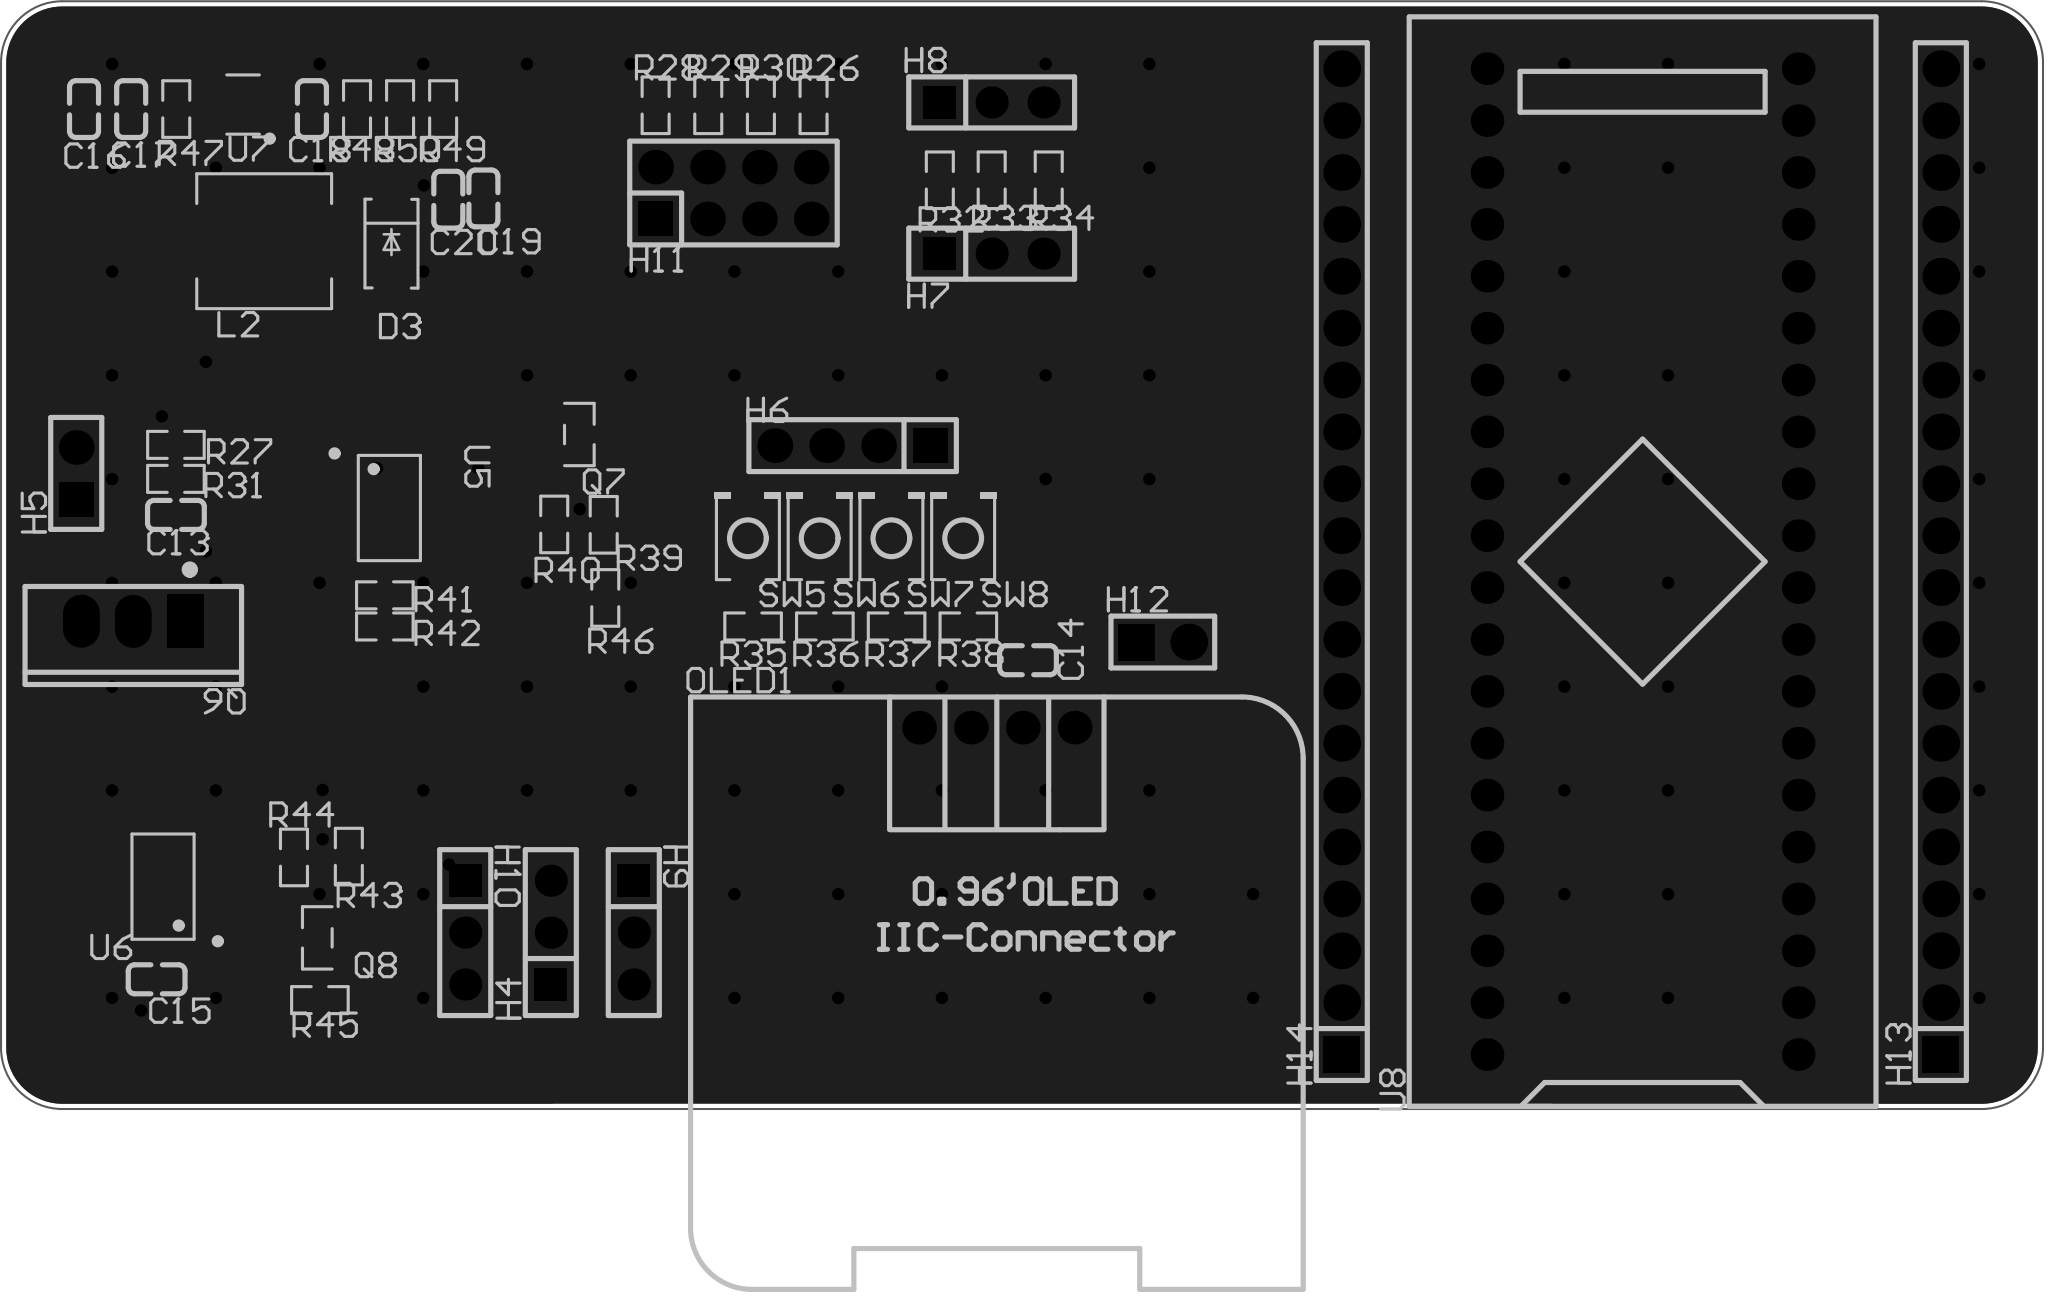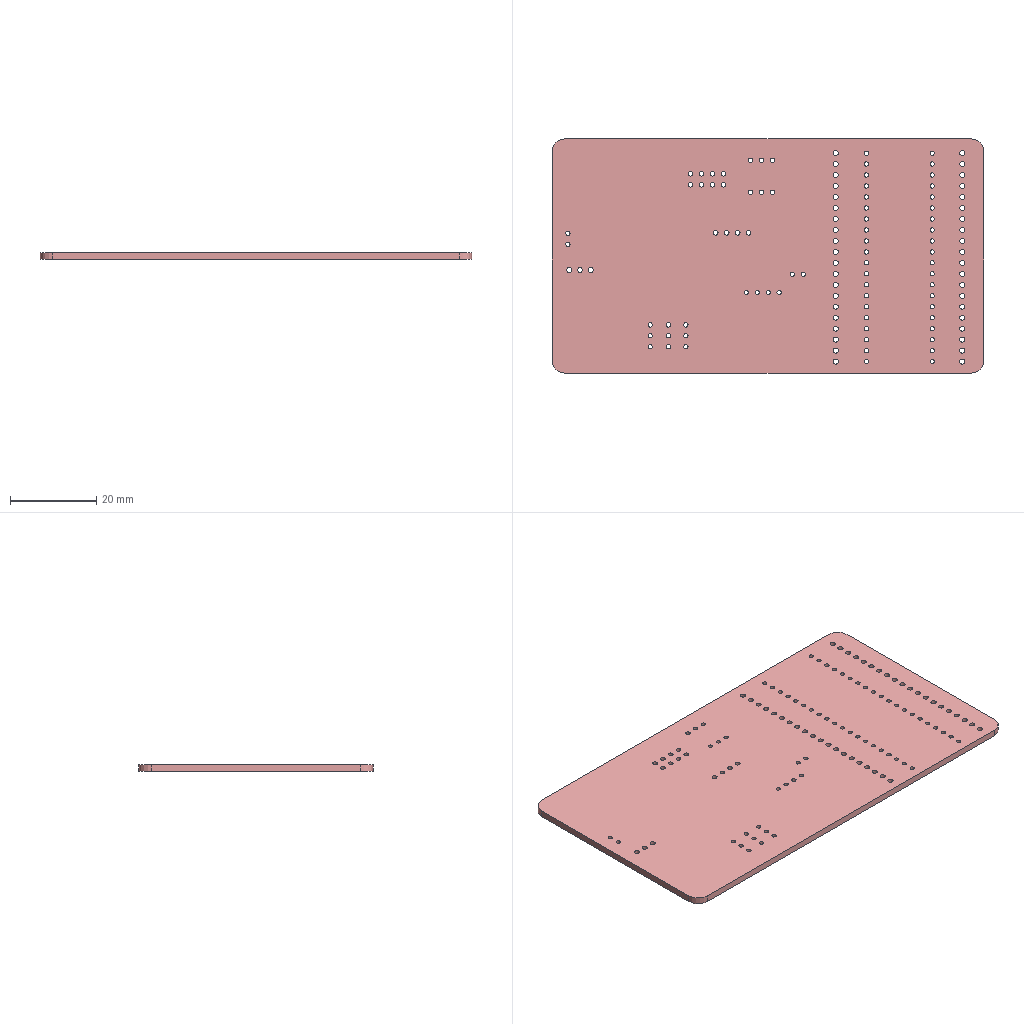Circuit board layout | Altium Designer | box 100 x 54.2 x 1.6 mm
Layer stack:
# Altium Designer layer stack of  (unit mm; dielectric type: 0 none, 1 core, 2 prepreg, 3 surface material)
index,name,kind,layer,copper_thickness_mm,dielectric_type,dielectric_thickness_mm,dielectric_material,dielectric_constant
0,Top Paste Mask Layer,other,,,,,,
1,Top Silkscreen Layer,other,,,,,,
2,Top Solder Mask Layer,dielectric,,,3,0.01,,3.3
3,Top Layer,copper,Top Layer,0.035,,,,
4,Dielectric1,dielectric,,,3,1.51,FR4,4.5
5,Bottom Layer,copper,Bottom Layer,0.035,,,,
6,Bottom Solder Mask Layer,dielectric,,,3,0.01,,3.3
7,Bottom Silkscreen Layer,other,,,,,,
8,Bottom Paste Mask Layer,other,,,,,,
# drill layer pairs: low layer,high layer
drill_pair,Top Layer,Bottom Layer
Part placement:
Designator,Comment,Layer,Footprint,Center-X(mm),Center-Y(mm),Rotation
C13,104,TopLayer,C0603,87.178,114.214,0
C14,10uf,TopLayer,C0603,128.905,107.102,180
C15,100nF,TopLayer,C0603,86.233,91.481,180
C16,106,TopLayer,C0603,82.677,134.082,90
C17,104,TopLayer,C0603,84.986,134.082,90
C18,100pF,TopLayer,C0603,93.838,134.082,90
C19,10UF,TopLayer,C0603,102.235,129.708,270
C20,104,TopLayer,C0603,100.517,129.645,270
D3,SS36,TopLayer,SMA_L4.3-W2.6-LS5.0-FD,97.723,127.487,90
H4,,TopLayer,HDR-TH_3P-P2.54-V-F,105.537,93.767,90
H5,,TopLayer,HDR-TH_2P-P2.54-V-F,82.296,116.246,90
H6,,TopLayer,HDR-TH_4P-P2.54-V-M,120.317,117.606,180
H7,,TopLayer,HDR-TH_3P-P2.54-V-F,127.127,127.004,0
H8,,TopLayer,HDR-TH_3P-P2.54-V-F,127.127,134.407,0
H9,,TopLayer,HDR-TH_3P-P2.54-V-F,109.601,93.767,270
H10,,TopLayer,HDR-TH_3P-P2.54-V-F,101.346,93.767,270
H11,,TopLayer,HDR-TH_8P-P2.54-V-M-R2-C4-S2.54,114.482,129.973,0
L2,22uH,TopLayer,IND-SMD_L7.1-W6.6,91.5,127.614,0
Q6,2N6804,TopLayer,TO-220-3_L10.0-W4.5-P2.54-L,85.09,109.007,180
Q7,SS8550,TopLayer,SOT-23-3_L2.9-W1.3-P1.90-LS2.4-BR,106.934,118.151,180
Q8,SS8550,TopLayer,SOT-23-3_L2.9-W1.3-P1.90-LS2.4-BR,94.102,93.509,0
R26,100K,TopLayer,R0603,118.404,134.267,90
R27,1K,TopLayer,R0603,87.178,117.643,180
R28,200,TopLayer,R0603,110.669,134.267,90
R29,2K,TopLayer,R0603,113.248,134.267,90
R30,20K,TopLayer,R0603,115.826,134.267,90
R31,1K,TopLayer,R0603,87.178,115.979,0
R32,100,TopLayer,R0603,124.587,130.597,270
R33,100,TopLayer,R0603,127.127,130.597,270
R34,100,TopLayer,R0603,129.921,130.597,90
R35,100,TopLayer,R0603,115.443,108.753,0
R36,100,TopLayer,R0603,118.957,108.753,0
R37,100,TopLayer,R0603,122.47,108.753,0
R38,100,TopLayer,R0603,125.984,108.753,0
R39,1K,TopLayer,R0603,108.127,113.731,90
R40,250K,TopLayer,R0603,105.704,113.748,90
R41,10K,TopLayer,R0603,97.409,110.277,180
R42,10K,TopLayer,R0603,97.409,108.753,0
R43,10K,TopLayer,R0603,95.646,97.487,90
R44,10K,TopLayer,R0603,92.959,97.446,270
R45,250K,TopLayer,R0603,94.229,90.461,0
R46,1K,TopLayer,R0603,108.204,110.15,270
R47,1K,TopLayer,R0603,87.195,134.082,270
R48,1K,TopLayer,R0603,96.047,134.082,90
R49,9.1K,TopLayer,R0603,100.263,134.082,90
R50,75K,TopLayer,R0603,98.155,134.082,90
SW5,TS-1088-AR02016,TopLayer,SW-SMD_L3.9-W3.0-P4.45,115.189,113.071,90
SW6,TS-1088-AR02016,TopLayer,SW-SMD_L3.9-W3.0-P4.45,118.703,113.071,90
SW7,TS-1088-AR02016,TopLayer,SW-SMD_L3.9-W3.0-P4.45,122.216,113.071,90
SW8,TS-1088-AR02016,TopLayer,SW-SMD_L3.9-W3.0-P4.45,125.73,113.071,90
U5,LM358DTR(XBLW),TopLayer,SOIC-8_L4.9-W4.0-P1.27-LS6.0-BL,97.63,114.552,270
U6,LM358DTR(XBLW),TopLayer,SOIC-8_L4.9-W4.0-P1.27-LS6.0-BL,86.546,96.017,90
U7,MT3608L,TopLayer,SOT-23-6_L2.9-W1.6-P0.95-LS2.8-BL_3,90.466,134.303,90
H12,,TopLayer,HDR-TH_2P-P2.54-V-M-1,135.509,107.991,0
U8,STM32F103C8T6-Card,TopLayer,CONN-TH_L53.3-W22.9_STM32F103C8T6-CARD,159.004,111.928,90
H13,,TopLayer,HDR-TH_20P-P2.54-V-M-1,173.609,111.928,90
H14,,TopLayer,HDR-TH_20P-P2.54-V-M-1,144.272,111.928,90
OLED1,,TopLayer,0.96OLED_4P,127.381,103.8,0
Pad and via stacks:
# Altium Designer via and pad stacks of  (unit mm). Each distinct definition once, with the count of objects using it.
# via: kind,start_layer,end_layer,hole_mm,diameter_mm,mode(0 simple;1 top-mid-bottom;2 full stack),diameter_per_layer,count,example_net
# pad: kind,layer,hole_mm,hole_type(0 round;1 square;2 slot),plating,top_size,top_shape(1 round;2 rect;3 octagon;9 rounded rect),mid_size,bottom_size,mode,footprint,size_per_layer,count,example
pad,Top Layer,0,0,plated,0.8x0.9,2,0.8x0.9,0.8x0.9,0,C0603,,16,C13.2
pad,Top Layer,0,0,plated,2.046x1.62,2,2.046x1.62,2.046x1.62,0,SMA_L4.3-W2.6-LS5.0-FD,,2,D3.1
pad,Top Layer,0,0,plated,2.15x3.32,2,2.15x3.32,2.15x3.32,0,IND-SMD_L7.1-W6.6,,2,L2.2
pad,Top Layer,0,0,plated,1.25x0.7,2,1.25x0.7,1.25x0.7,0,SOT-23-3_L2.9-W1.3-P1.90-LS2.4-BR,,6,Q7.1
pad,Top Layer,0,0,plated,0.8065x0.864,2,0.8065x0.864,0.8065x0.864,0,R0603,,50,R26.2
pad,Top Layer,0,0,plated,1.23x1.36,2,1.23x1.36,1.23x1.36,0,SW-SMD_L3.9-W3.0-P4.45,,8,SW5.1
pad,Top Layer,0,0,plated,0.63x1.865,1,0.63x1.865,0.63x1.865,0,SOIC-8_L4.9-W4.0-P1.27-LS6.0-BL,,16,U5.1
pad,Top Layer,0,0,plated,0.6x1.2,2,0.6x1.2,0.6x1.2,0,SOT-23-6_L2.9-W1.6-P0.95-LS2.8-BL_3,,6,U7.6
pad,Multi-Layer,1.02,0,plated,1.575x1.575,1,1.575x1.575,1.575x1.575,0,HDR-TH_3P-P2.54-V-F,,10,H4.3
pad,Multi-Layer,1.02,0,plated,1.575x1.575,2,1.575x1.575,1.575x1.575,0,HDR-TH_3P-P2.54-V-F,,5,H4.1
pad,Multi-Layer,1,0,plated,1.7x1.7,2,1.7x1.7,1.7x1.7,0,HDR-TH_2P-P2.54-V-F,,1,H5.1
pad,Multi-Layer,1,0,plated,1.7x1.7,1,1.7x1.7,1.7x1.7,0,HDR-TH_2P-P2.54-V-F,,1,H5.2
pad,Multi-Layer,1.1,0,plated,1.7x1.7,2,1.7x1.7,1.7x1.7,0,HDR-TH_4P-P2.54-V-M,,1,H6.1
pad,Multi-Layer,1.1,0,plated,1.7x1.7,1,1.7x1.7,1.7x1.7,0,HDR-TH_4P-P2.54-V-M,,3,H6.2
pad,Multi-Layer,1.1,0,plated,1.7x1.7,2,1.7x1.7,1.7x1.7,0,HDR-TH_8P-P2.54-V-M-R2-C4-S2.54,,1,H11.1
pad,Multi-Layer,1.1,0,plated,1.7x1.7,1,1.7x1.7,1.7x1.7,0,HDR-TH_8P-P2.54-V-M-R2-C4-S2.54,,7,H11.2
pad,Multi-Layer,1.2,0,plated,1.8x2.6,1,1.8x2.6,1.8x2.6,0,TO-220-3_L10.0-W4.5-P2.54-L,,2,Q6.2
pad,Multi-Layer,1.2,0,plated,1.8x2.6,2,1.8x2.6,1.8x2.6,0,TO-220-3_L10.0-W4.5-P2.54-L,,1,Q6.1
pad,Multi-Layer,1,0,plated,1.8x1.8,1,1.8x1.8,1.8x1.8,0,HDR-TH_2P-P2.54-V-M-1,,1,H12.2
pad,Multi-Layer,1,0,plated,1.8x1.8,2,1.8x1.8,1.8x1.8,0,HDR-TH_2P-P2.54-V-M-1,,1,H12.1
pad,Multi-Layer,1,0,plated,1.6x1.6,1,1.6x1.6,1.6x1.6,0,CONN-TH_L53.3-W22.9_STM32F103C8T6-CARD,,40,U8.1
pad,Multi-Layer,1.2,0,plated,1.8x1.8,1,1.8x1.8,1.8x1.8,0,HDR-TH_20P-P2.54-V-M-1,,38,H13.20
pad,Multi-Layer,1.2,0,plated,1.8x1.8,2,1.8x1.8,1.8x1.8,0,HDR-TH_20P-P2.54-V-M-1,,2,H13.1
pad,Multi-Layer,1,0,plated,1.65x1.65,1,1.65x1.65,1.65x1.65,0,0.96OLED_4P,,4,OLED1.4
via,Top Layer,Bottom Layer,0.3048,0.61,0,,113,$1N17
Copper pours:
name,layer,net,type(0 solid;1 hatched;2 none)
Top Layer-GND,Top Layer,GND,0
Bottom Layer-GND,Bottom Layer,GND,0